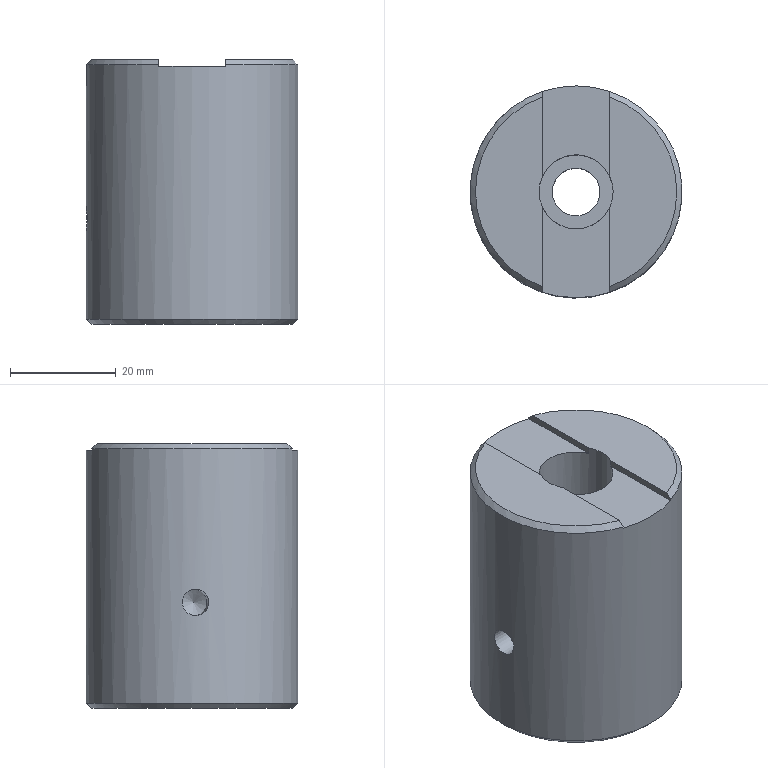Part | STEP file | gslz 2016.10.28-6_id170_x_t | 1 solid | 18 faces | box 40 x 40 x 50 mm | volume 56993 mm3 | plane 10 | cylinder 4 | cone 4 | commonest cylinder face diameters 5 x1 9 x1 14 x1 40 x1
STEP:
#1=CARTESIAN_POINT('',(-259.,150.,-0.007538));
#2=VERTEX_POINT('',#1);
#3=CARTESIAN_POINT('',(-240.,150.,-0.007538));
#4=DIRECTION('',(0.,0.,1.));
#5=DIRECTION('',(-1.,0.,0.));
#6=AXIS2_PLACEMENT_3D('',#3,#4,#5);
#7=CIRCLE('',#6,19.);
#8=EDGE_CURVE('',#2,#2,#7,.T.);
#9=ORIENTED_EDGE('',*,*,#8,.F.);
#10=EDGE_LOOP('',(#9));
#11=FACE_BOUND('',#10,.T.);
#12=CARTESIAN_POINT('',(-235.5,150.,-0.007538));
#13=VERTEX_POINT('',#12);
#14=CARTESIAN_POINT('',(-240.,150.,-0.007538));
#15=DIRECTION('',(0.,0.,1.));
#16=DIRECTION('',(1.,0.,0.));
#17=AXIS2_PLACEMENT_3D('',#14,#15,#16);
#18=CIRCLE('',#17,4.5);
#19=EDGE_CURVE('',#13,#13,#18,.T.);
#20=ORIENTED_EDGE('',*,*,#19,.T.);
#21=EDGE_LOOP('',(#20));
#22=FACE_BOUND('',#21,.T.);
#23=CARTESIAN_POINT('',(-240.,150.,-0.007538));
#24=DIRECTION('',(0.,0.,1.));
#25=DIRECTION('',(-1.,0.,0.));
#26=AXIS2_PLACEMENT_3D('',#23,#24,#25);
#27=PLANE('',#26);
#28=ADVANCED_FACE('',(#11,#22),#27,.F.);
#29=CARTESIAN_POINT('',(-233.65,147.054,49.992));
#30=VERTEX_POINT('',#29);
#31=CARTESIAN_POINT('',(-233.65,132.093,49.992));
#32=VERTEX_POINT('',#31);
#33=CARTESIAN_POINT('',(-233.65,150.,49.992));
#34=DIRECTION('',(0.,-1.,0.));
#35=VECTOR('',#34,1.);
#36=LINE('',#33,#35);
#37=EDGE_CURVE('',#30,#32,#36,.T.);
#38=ORIENTED_EDGE('',*,*,#37,.T.);
#39=CARTESIAN_POINT('',(-233.65,167.907,49.992));
#40=VERTEX_POINT('',#39);
#41=CARTESIAN_POINT('',(-240.,150.,49.992));
#42=DIRECTION('',(0.,0.,-1.));
#43=DIRECTION('',(-1.,0.,0.));
#44=AXIS2_PLACEMENT_3D('',#41,#42,#43);
#45=CIRCLE('',#44,19.);
#46=EDGE_CURVE('',#40,#32,#45,.T.);
#47=ORIENTED_EDGE('',*,*,#46,.F.);
#48=CARTESIAN_POINT('',(-233.65,152.946,49.992));
#49=VERTEX_POINT('',#48);
#50=CARTESIAN_POINT('',(-233.65,150.,49.992));
#51=DIRECTION('',(0.,-1.,0.));
#52=VECTOR('',#51,1.);
#53=LINE('',#50,#52);
#54=EDGE_CURVE('',#40,#49,#53,.T.);
#55=ORIENTED_EDGE('',*,*,#54,.T.);
#56=CARTESIAN_POINT('',(-240.,150.,49.992));
#57=DIRECTION('',(0.,0.,1.));
#58=DIRECTION('',(1.,0.,0.));
#59=AXIS2_PLACEMENT_3D('',#56,#57,#58);
#60=CIRCLE('',#59,7.);
#61=EDGE_CURVE('',#30,#49,#60,.T.);
#62=ORIENTED_EDGE('',*,*,#61,.F.);
#63=EDGE_LOOP('',(#38,#47,#55,#62));
#64=FACE_OUTER_BOUND('',#63,.T.);
#65=CARTESIAN_POINT('',(-240.,150.,49.992));
#66=DIRECTION('',(0.,0.,1.));
#67=DIRECTION('',(-1.,0.,0.));
#68=AXIS2_PLACEMENT_3D('',#65,#66,#67);
#69=PLANE('',#68);
#70=ADVANCED_FACE('',(#64),#69,.T.);
#71=CARTESIAN_POINT('',(-246.35,152.946,49.992));
#72=VERTEX_POINT('',#71);
#73=CARTESIAN_POINT('',(-246.35,167.907,49.992));
#74=VERTEX_POINT('',#73);
#75=CARTESIAN_POINT('',(-246.35,150.,49.992));
#76=DIRECTION('',(0.,1.,0.));
#77=VECTOR('',#76,1.);
#78=LINE('',#75,#77);
#79=EDGE_CURVE('',#72,#74,#78,.T.);
#80=ORIENTED_EDGE('',*,*,#79,.T.);
#81=CARTESIAN_POINT('',(-246.35,132.093,49.992));
#82=VERTEX_POINT('',#81);
#83=CARTESIAN_POINT('',(-240.,150.,49.992));
#84=DIRECTION('',(0.,0.,-1.));
#85=DIRECTION('',(-1.,0.,0.));
#86=AXIS2_PLACEMENT_3D('',#83,#84,#85);
#87=CIRCLE('',#86,19.);
#88=EDGE_CURVE('',#82,#74,#87,.T.);
#89=ORIENTED_EDGE('',*,*,#88,.F.);
#90=CARTESIAN_POINT('',(-246.35,147.054,49.992));
#91=VERTEX_POINT('',#90);
#92=CARTESIAN_POINT('',(-246.35,150.,49.992));
#93=DIRECTION('',(0.,1.,0.));
#94=VECTOR('',#93,1.);
#95=LINE('',#92,#94);
#96=EDGE_CURVE('',#82,#91,#95,.T.);
#97=ORIENTED_EDGE('',*,*,#96,.T.);
#98=CARTESIAN_POINT('',(-240.,150.,49.992));
#99=DIRECTION('',(0.,0.,1.));
#100=DIRECTION('',(1.,0.,0.));
#101=AXIS2_PLACEMENT_3D('',#98,#99,#100);
#102=CIRCLE('',#101,7.);
#103=EDGE_CURVE('',#72,#91,#102,.T.);
#104=ORIENTED_EDGE('',*,*,#103,.F.);
#105=EDGE_LOOP('',(#80,#89,#97,#104));
#106=FACE_OUTER_BOUND('',#105,.T.);
#107=CARTESIAN_POINT('',(-240.,150.,49.992));
#108=DIRECTION('',(0.,0.,1.));
#109=DIRECTION('',(-1.,0.,0.));
#110=AXIS2_PLACEMENT_3D('',#107,#108,#109);
#111=PLANE('',#110);
#112=ADVANCED_FACE('',(#106),#111,.T.);
#113=ORIENTED_EDGE('',*,*,#96,.F.);
#114=CARTESIAN_POINT('',(-246.35,131.035,48.992));
#115=VERTEX_POINT('',#114);
#116=CARTESIAN_POINT('',(-246.35,131.035,48.992));
#117=CARTESIAN_POINT('',(-246.35,131.387,49.326));
#118=CARTESIAN_POINT('',(-246.35,131.739,49.66));
#119=CARTESIAN_POINT('',(-246.35,132.093,49.992));
#120=B_SPLINE_CURVE_WITH_KNOTS('',3,(#116,#117,#118,#119),.UNSPECIFIED.,.F.,.F.,(4,4),(0.,1.),.UNSPECIFIED.);
#121=EDGE_CURVE('',#115,#82,#120,.T.);
#122=ORIENTED_EDGE('',*,*,#121,.F.);
#123=CARTESIAN_POINT('',(-246.35,131.035,48.722));
#124=VERTEX_POINT('',#123);
#125=CARTESIAN_POINT('',(-246.35,131.035,-35.008));
#126=DIRECTION('',(0.,0.,1.));
#127=VECTOR('',#126,1.);
#128=LINE('',#125,#127);
#129=EDGE_CURVE('',#124,#115,#128,.T.);
#130=ORIENTED_EDGE('',*,*,#129,.F.);
#131=CARTESIAN_POINT('',(-246.35,147.054,48.722));
#132=VERTEX_POINT('',#131);
#133=CARTESIAN_POINT('',(-246.35,1261.518,48.722));
#134=DIRECTION('',(0.,1.,0.));
#135=VECTOR('',#134,1.);
#136=LINE('',#133,#135);
#137=EDGE_CURVE('',#124,#132,#136,.T.);
#138=ORIENTED_EDGE('',*,*,#137,.T.);
#139=CARTESIAN_POINT('',(-246.35,147.054,39.992));
#140=DIRECTION('',(0.,0.,-1.));
#141=VECTOR('',#140,1.);
#142=LINE('',#139,#141);
#143=EDGE_CURVE('',#91,#132,#142,.T.);
#144=ORIENTED_EDGE('',*,*,#143,.F.);
#145=EDGE_LOOP('',(#113,#122,#130,#138,#144));
#146=FACE_OUTER_BOUND('',#145,.T.);
#147=CARTESIAN_POINT('',(-246.35,1261.518,124.992));
#148=DIRECTION('',(-1.,0.,0.));
#149=DIRECTION('',(0.,0.,-1.));
#150=AXIS2_PLACEMENT_3D('',#147,#148,#149);
#151=PLANE('',#150);
#152=ADVANCED_FACE('',(#146),#151,.F.);
#153=ORIENTED_EDGE('',*,*,#54,.F.);
#154=CARTESIAN_POINT('',(-233.65,168.965,48.992));
#155=VERTEX_POINT('',#154);
#156=CARTESIAN_POINT('',(-233.65,168.965,48.992));
#157=CARTESIAN_POINT('',(-233.65,168.613,49.326));
#158=CARTESIAN_POINT('',(-233.65,168.261,49.66));
#159=CARTESIAN_POINT('',(-233.65,167.907,49.992));
#160=B_SPLINE_CURVE_WITH_KNOTS('',3,(#156,#157,#158,#159),.UNSPECIFIED.,.F.,.F.,(4,4),(0.,1.),.UNSPECIFIED.);
#161=EDGE_CURVE('',#155,#40,#160,.T.);
#162=ORIENTED_EDGE('',*,*,#161,.F.);
#163=CARTESIAN_POINT('',(-233.65,168.965,48.722));
#164=VERTEX_POINT('',#163);
#165=CARTESIAN_POINT('',(-233.65,168.965,-35.008));
#166=DIRECTION('',(0.,0.,1.));
#167=VECTOR('',#166,1.);
#168=LINE('',#165,#167);
#169=EDGE_CURVE('',#164,#155,#168,.T.);
#170=ORIENTED_EDGE('',*,*,#169,.F.);
#171=CARTESIAN_POINT('',(-233.65,152.946,48.722));
#172=VERTEX_POINT('',#171);
#173=CARTESIAN_POINT('',(-233.65,-113.507,48.722));
#174=DIRECTION('',(0.,-1.,0.));
#175=VECTOR('',#174,1.);
#176=LINE('',#173,#175);
#177=EDGE_CURVE('',#164,#172,#176,.T.);
#178=ORIENTED_EDGE('',*,*,#177,.T.);
#179=CARTESIAN_POINT('',(-233.65,152.946,39.992));
#180=DIRECTION('',(0.,0.,-1.));
#181=VECTOR('',#180,1.);
#182=LINE('',#179,#181);
#183=EDGE_CURVE('',#49,#172,#182,.T.);
#184=ORIENTED_EDGE('',*,*,#183,.F.);
#185=EDGE_LOOP('',(#153,#162,#170,#178,#184));
#186=FACE_OUTER_BOUND('',#185,.T.);
#187=CARTESIAN_POINT('',(-233.65,-113.507,124.992));
#188=DIRECTION('',(1.,0.,0.));
#189=DIRECTION('',(0.,0.,1.));
#190=AXIS2_PLACEMENT_3D('',#187,#188,#189);
#191=PLANE('',#190);
#192=ADVANCED_FACE('',(#186),#191,.F.);
#193=CARTESIAN_POINT('',(-246.35,152.946,48.722));
#194=VERTEX_POINT('',#193);
#195=CARTESIAN_POINT('',(-240.,150.,48.722));
#196=DIRECTION('',(0.,0.,-1.));
#197=DIRECTION('',(-1.,0.,0.));
#198=AXIS2_PLACEMENT_3D('',#195,#196,#197);
#199=CIRCLE('',#198,7.);
#200=EDGE_CURVE('',#194,#172,#199,.T.);
#201=ORIENTED_EDGE('',*,*,#200,.T.);
#202=ORIENTED_EDGE('',*,*,#177,.F.);
#203=CARTESIAN_POINT('',(-246.35,168.965,48.722));
#204=VERTEX_POINT('',#203);
#205=CARTESIAN_POINT('',(-240.,150.,48.722));
#206=DIRECTION('',(0.,0.,1.));
#207=DIRECTION('',(-1.,0.,0.));
#208=AXIS2_PLACEMENT_3D('',#205,#206,#207);
#209=CIRCLE('',#208,20.);
#210=EDGE_CURVE('',#164,#204,#209,.T.);
#211=ORIENTED_EDGE('',*,*,#210,.T.);
#212=CARTESIAN_POINT('',(-246.35,1261.518,48.722));
#213=DIRECTION('',(0.,1.,0.));
#214=VECTOR('',#213,1.);
#215=LINE('',#212,#214);
#216=EDGE_CURVE('',#194,#204,#215,.T.);
#217=ORIENTED_EDGE('',*,*,#216,.F.);
#218=EDGE_LOOP('',(#201,#202,#211,#217));
#219=FACE_OUTER_BOUND('',#218,.T.);
#220=CARTESIAN_POINT('',(-233.65,574.005,48.722));
#221=DIRECTION('',(0.,0.,1.));
#222=DIRECTION('',(-1.,0.,0.));
#223=AXIS2_PLACEMENT_3D('',#220,#221,#222);
#224=PLANE('',#223);
#225=ADVANCED_FACE('',(#219),#224,.T.);
#226=CARTESIAN_POINT('',(-260.,150.,0.9925));
#227=VERTEX_POINT('',#226);
#228=CARTESIAN_POINT('',(-240.,150.,0.9925));
#229=DIRECTION('',(0.,0.,-1.));
#230=DIRECTION('',(-1.,0.,0.));
#231=AXIS2_PLACEMENT_3D('',#228,#229,#230);
#232=CIRCLE('',#231,20.);
#233=EDGE_CURVE('',#227,#227,#232,.T.);
#234=ORIENTED_EDGE('',*,*,#233,.F.);
#235=EDGE_LOOP('',(#234));
#236=FACE_BOUND('',#235,.T.);
#237=CARTESIAN_POINT('',(-233.65,131.035,48.992));
#238=VERTEX_POINT('',#237);
#239=CARTESIAN_POINT('',(-233.65,131.035,48.722));
#240=VERTEX_POINT('',#239);
#241=CARTESIAN_POINT('',(-233.65,131.035,-35.008));
#242=DIRECTION('',(0.,0.,-1.));
#243=VECTOR('',#242,1.);
#244=LINE('',#241,#243);
#245=EDGE_CURVE('',#238,#240,#244,.T.);
#246=ORIENTED_EDGE('',*,*,#245,.T.);
#247=CARTESIAN_POINT('',(-240.,150.,48.722));
#248=DIRECTION('',(0.,0.,1.));
#249=DIRECTION('',(-1.,0.,0.));
#250=AXIS2_PLACEMENT_3D('',#247,#248,#249);
#251=CIRCLE('',#250,20.);
#252=EDGE_CURVE('',#124,#240,#251,.T.);
#253=ORIENTED_EDGE('',*,*,#252,.F.);
#254=ORIENTED_EDGE('',*,*,#129,.T.);
#255=CARTESIAN_POINT('',(-246.35,168.965,48.992));
#256=VERTEX_POINT('',#255);
#257=CARTESIAN_POINT('',(-240.,150.,48.992));
#258=DIRECTION('',(0.,0.,1.));
#259=DIRECTION('',(-1.,0.,0.));
#260=AXIS2_PLACEMENT_3D('',#257,#258,#259);
#261=CIRCLE('',#260,20.);
#262=EDGE_CURVE('',#256,#115,#261,.T.);
#263=ORIENTED_EDGE('',*,*,#262,.F.);
#264=CARTESIAN_POINT('',(-246.35,168.965,48.857));
#265=DIRECTION('',(0.,0.,-1.));
#266=VECTOR('',#265,1.);
#267=LINE('',#264,#266);
#268=EDGE_CURVE('',#256,#204,#267,.T.);
#269=ORIENTED_EDGE('',*,*,#268,.T.);
#270=ORIENTED_EDGE('',*,*,#210,.F.);
#271=ORIENTED_EDGE('',*,*,#169,.T.);
#272=CARTESIAN_POINT('',(-240.,150.,48.992));
#273=DIRECTION('',(0.,0.,1.));
#274=DIRECTION('',(-1.,0.,0.));
#275=AXIS2_PLACEMENT_3D('',#272,#273,#274);
#276=CIRCLE('',#275,20.);
#277=EDGE_CURVE('',#238,#155,#276,.T.);
#278=ORIENTED_EDGE('',*,*,#277,.F.);
#279=EDGE_LOOP('',(#246,#253,#254,#263,#269,#270,#271,#278));
#280=FACE_BOUND('',#279,.T.);
#281=CARTESIAN_POINT('',(-259.98,149.117,17.502));
#282=VERTEX_POINT('',#281);
#283=CARTESIAN_POINT('',(-259.98,149.117,17.502));
#284=CARTESIAN_POINT('',(-259.993,149.394,17.478));
#285=CARTESIAN_POINT('',(-259.999,149.679,17.5));
#286=CARTESIAN_POINT('',(-260.,149.949,17.568));
#287=CARTESIAN_POINT('',(-260.001,150.218,17.637));
#288=CARTESIAN_POINT('',(-259.996,150.48,17.752));
#289=CARTESIAN_POINT('',(-259.987,150.713,17.904));
#290=CARTESIAN_POINT('',(-259.979,150.946,18.058));
#291=CARTESIAN_POINT('',(-259.967,151.156,18.253));
#292=CARTESIAN_POINT('',(-259.956,151.326,18.475));
#293=CARTESIAN_POINT('',(-259.945,151.496,18.698));
#294=CARTESIAN_POINT('',(-259.934,151.631,18.953));
#295=CARTESIAN_POINT('',(-259.926,151.718,19.22));
#296=CARTESIAN_POINT('',(-259.919,151.805,19.486));
#297=CARTESIAN_POINT('',(-259.915,151.847,19.771));
#298=CARTESIAN_POINT('',(-259.915,151.84,20.051));
#299=CARTESIAN_POINT('',(-259.916,151.834,20.328));
#300=CARTESIAN_POINT('',(-259.921,151.779,20.609));
#301=CARTESIAN_POINT('',(-259.929,151.681,20.869));
#302=CARTESIAN_POINT('',(-259.937,151.584,21.129));
#303=CARTESIAN_POINT('',(-259.949,151.44,21.376));
#304=CARTESIAN_POINT('',(-259.96,151.262,21.59));
#305=CARTESIAN_POINT('',(-259.971,151.083,21.805));
#306=CARTESIAN_POINT('',(-259.983,150.864,21.992));
#307=CARTESIAN_POINT('',(-259.99,150.624,22.136));
#308=CARTESIAN_POINT('',(-259.998,150.384,22.28));
#309=CARTESIAN_POINT('',(-260.002,150.114,22.385));
#310=CARTESIAN_POINT('',(-259.999,149.839,22.441));
#311=CARTESIAN_POINT('',(-259.997,149.566,22.498));
#312=CARTESIAN_POINT('',(-259.989,149.279,22.507));
#313=CARTESIAN_POINT('',(-259.975,149.003,22.47));
#314=CARTESIAN_POINT('',(-259.961,148.728,22.433));
#315=CARTESIAN_POINT('',(-259.942,148.456,22.348));
#316=CARTESIAN_POINT('',(-259.92,148.209,22.223));
#317=CARTESIAN_POINT('',(-259.897,147.961,22.097));
#318=CARTESIAN_POINT('',(-259.872,147.732,21.927));
#319=CARTESIAN_POINT('',(-259.848,147.54,21.727));
#320=CARTESIAN_POINT('',(-259.824,147.346,21.525));
#321=CARTESIAN_POINT('',(-259.801,147.185,21.287));
#322=CARTESIAN_POINT('',(-259.784,147.069,21.032));
#323=CARTESIAN_POINT('',(-259.767,146.953,20.777));
#324=CARTESIAN_POINT('',(-259.755,146.879,20.498));
#325=CARTESIAN_POINT('',(-259.751,146.854,20.219));
#326=CARTESIAN_POINT('',(-259.747,146.829,19.942));
#327=CARTESIAN_POINT('',(-259.751,146.851,19.656));
#328=CARTESIAN_POINT('',(-259.761,146.918,19.386));
#329=CARTESIAN_POINT('',(-259.771,146.985,19.117));
#330=CARTESIAN_POINT('',(-259.789,147.099,18.855));
#331=CARTESIAN_POINT('',(-259.81,147.25,18.623));
#332=CARTESIAN_POINT('',(-259.831,147.402,18.39));
#333=CARTESIAN_POINT('',(-259.856,147.596,18.18));
#334=CARTESIAN_POINT('',(-259.88,147.817,18.01));
#335=CARTESIAN_POINT('',(-259.905,148.038,17.839));
#336=CARTESIAN_POINT('',(-259.929,148.293,17.704));
#337=CARTESIAN_POINT('',(-259.948,148.559,17.617));
#338=CARTESIAN_POINT('',(-259.961,148.739,17.558));
#339=CARTESIAN_POINT('',(-259.972,148.927,17.519));
#340=CARTESIAN_POINT('',(-259.98,149.117,17.502));
#341=B_SPLINE_CURVE_WITH_KNOTS('',3,(#283,#284,#285,#286,#287,#288,#289,#290,#291,#292,#293,#294,#295,#296,#297,#298,#299,#300,#301,#302,#303,#304,#305,#306,#307,#308,#309,#310,#311,#312,#313,#314,#315,#316,#317,#318,#319,#320,#321,#322,#323,#324,#325,#326,#327,#328,#329,#330,#331,#332,#333,#334,#335,#336,#337,#338,#339,#340),.UNSPECIFIED.,.T.,.F.,(1,3,3,3,3,3,3,3,3,3,3,3,3,3,3,3,3,3,3,3,3,1),(-0.0362,0.,0.05335,0.1067,0.1602,0.2141,0.2678,0.3211,0.3744,0.4281,0.4819,0.5355,0.5887,0.6421,0.6959,0.7497,0.8031,0.8564,0.9099,0.9638,1.,1.053),.UNSPECIFIED.);
#342=EDGE_CURVE('',#282,#282,#341,.T.);
#343=ORIENTED_EDGE('',*,*,#342,.T.);
#344=EDGE_LOOP('',(#343));
#345=FACE_BOUND('',#344,.T.);
#346=CARTESIAN_POINT('',(-240.,150.,-35.008));
#347=DIRECTION('',(0.,0.,1.));
#348=DIRECTION('',(1.,0.,0.));
#349=AXIS2_PLACEMENT_3D('',#346,#347,#348);
#350=CYLINDRICAL_SURFACE('',#349,20.);
#351=ADVANCED_FACE('',(#236,#280,#345),#350,.T.);
#352=ORIENTED_EDGE('',*,*,#216,.T.);
#353=ORIENTED_EDGE('',*,*,#268,.F.);
#354=CARTESIAN_POINT('',(-246.35,167.907,49.992));
#355=CARTESIAN_POINT('',(-246.35,168.261,49.66));
#356=CARTESIAN_POINT('',(-246.35,168.613,49.326));
#357=CARTESIAN_POINT('',(-246.35,168.965,48.992));
#358=B_SPLINE_CURVE_WITH_KNOTS('',3,(#354,#355,#356,#357),.UNSPECIFIED.,.F.,.F.,(4,4),(0.,1.),.UNSPECIFIED.);
#359=EDGE_CURVE('',#74,#256,#358,.T.);
#360=ORIENTED_EDGE('',*,*,#359,.F.);
#361=ORIENTED_EDGE('',*,*,#79,.F.);
#362=CARTESIAN_POINT('',(-246.35,152.946,39.992));
#363=DIRECTION('',(0.,0.,1.));
#364=VECTOR('',#363,1.);
#365=LINE('',#362,#364);
#366=EDGE_CURVE('',#194,#72,#365,.T.);
#367=ORIENTED_EDGE('',*,*,#366,.F.);
#368=EDGE_LOOP('',(#352,#353,#360,#361,#367));
#369=FACE_OUTER_BOUND('',#368,.T.);
#370=CARTESIAN_POINT('',(-246.35,1261.518,124.992));
#371=DIRECTION('',(-1.,0.,0.));
#372=DIRECTION('',(0.,0.,-1.));
#373=AXIS2_PLACEMENT_3D('',#370,#371,#372);
#374=PLANE('',#373);
#375=ADVANCED_FACE('',(#369),#374,.F.);
#376=CARTESIAN_POINT('',(-233.65,147.054,48.722));
#377=VERTEX_POINT('',#376);
#378=CARTESIAN_POINT('',(-233.65,-113.507,48.722));
#379=DIRECTION('',(0.,-1.,0.));
#380=VECTOR('',#379,1.);
#381=LINE('',#378,#380);
#382=EDGE_CURVE('',#377,#240,#381,.T.);
#383=ORIENTED_EDGE('',*,*,#382,.T.);
#384=ORIENTED_EDGE('',*,*,#245,.F.);
#385=CARTESIAN_POINT('',(-233.65,132.093,49.992));
#386=CARTESIAN_POINT('',(-233.65,131.739,49.66));
#387=CARTESIAN_POINT('',(-233.65,131.387,49.326));
#388=CARTESIAN_POINT('',(-233.65,131.035,48.992));
#389=B_SPLINE_CURVE_WITH_KNOTS('',3,(#385,#386,#387,#388),.UNSPECIFIED.,.F.,.F.,(4,4),(0.,1.),.UNSPECIFIED.);
#390=EDGE_CURVE('',#32,#238,#389,.T.);
#391=ORIENTED_EDGE('',*,*,#390,.F.);
#392=ORIENTED_EDGE('',*,*,#37,.F.);
#393=CARTESIAN_POINT('',(-233.65,147.054,39.992));
#394=DIRECTION('',(0.,0.,1.));
#395=VECTOR('',#394,1.);
#396=LINE('',#393,#395);
#397=EDGE_CURVE('',#377,#30,#396,.T.);
#398=ORIENTED_EDGE('',*,*,#397,.F.);
#399=EDGE_LOOP('',(#383,#384,#391,#392,#398));
#400=FACE_OUTER_BOUND('',#399,.T.);
#401=CARTESIAN_POINT('',(-233.65,-113.507,124.992));
#402=DIRECTION('',(1.,0.,0.));
#403=DIRECTION('',(0.,0.,1.));
#404=AXIS2_PLACEMENT_3D('',#401,#402,#403);
#405=PLANE('',#404);
#406=ADVANCED_FACE('',(#400),#405,.F.);
#407=CARTESIAN_POINT('',(-240.,150.,48.722));
#408=DIRECTION('',(0.,0.,-1.));
#409=DIRECTION('',(-1.,0.,0.));
#410=AXIS2_PLACEMENT_3D('',#407,#408,#409);
#411=CIRCLE('',#410,7.);
#412=EDGE_CURVE('',#377,#132,#411,.T.);
#413=ORIENTED_EDGE('',*,*,#412,.T.);
#414=ORIENTED_EDGE('',*,*,#137,.F.);
#415=ORIENTED_EDGE('',*,*,#252,.T.);
#416=ORIENTED_EDGE('',*,*,#382,.F.);
#417=EDGE_LOOP('',(#413,#414,#415,#416));
#418=FACE_OUTER_BOUND('',#417,.T.);
#419=CARTESIAN_POINT('',(-233.65,574.005,48.722));
#420=DIRECTION('',(0.,0.,1.));
#421=DIRECTION('',(-1.,0.,0.));
#422=AXIS2_PLACEMENT_3D('',#419,#420,#421);
#423=PLANE('',#422);
#424=ADVANCED_FACE('',(#418),#423,.T.);
#425=CARTESIAN_POINT('',(-249.912,147.17,19.992));
#426=VERTEX_POINT('',#425);
#427=CARTESIAN_POINT('',(-249.994,149.668,19.992));
#428=DIRECTION('',(0.9995,0.03316,0.));
#429=DIRECTION('',(0.03316,-0.9995,0.));
#430=AXIS2_PLACEMENT_3D('',#427,#428,#429);
#431=CIRCLE('',#430,2.5);
#432=EDGE_CURVE('',#426,#426,#431,.T.);
#433=ORIENTED_EDGE('',*,*,#432,.F.);
#434=EDGE_LOOP('',(#433));
#435=FACE_BOUND('',#434,.T.);
#436=CARTESIAN_POINT('',(-248.493,149.718,19.992));
#437=VERTEX_POINT('',#436);
#438=VERTEX_LOOP('',#437);
#439=FACE_BOUND('',#438,.T.);
#440=CARTESIAN_POINT('',(-249.994,149.668,19.992));
#441=DIRECTION('',(-0.9995,-0.03316,0.));
#442=DIRECTION('',(-0.03316,0.9995,0.));
#443=AXIS2_PLACEMENT_3D('',#440,#441,#442);
#444=CONICAL_SURFACE('',#443,2.5,59.);
#445=ADVANCED_FACE('',(#435,#439),#444,.F.);
#446=ORIENTED_EDGE('',*,*,#342,.F.);
#447=EDGE_LOOP('',(#446));
#448=FACE_BOUND('',#447,.T.);
#449=ORIENTED_EDGE('',*,*,#432,.T.);
#450=EDGE_LOOP('',(#449));
#451=FACE_BOUND('',#450,.T.);
#452=CARTESIAN_POINT('',(-264.986,149.171,19.992));
#453=DIRECTION('',(0.9995,0.03316,0.));
#454=DIRECTION('',(-0.03316,0.9995,0.));
#455=AXIS2_PLACEMENT_3D('',#452,#453,#454);
#456=CYLINDRICAL_SURFACE('',#455,2.5);
#457=ADVANCED_FACE('',(#448,#451),#456,.F.);
#458=ORIENTED_EDGE('',*,*,#8,.T.);
#459=EDGE_LOOP('',(#458));
#460=FACE_BOUND('',#459,.T.);
#461=ORIENTED_EDGE('',*,*,#233,.T.);
#462=EDGE_LOOP('',(#461));
#463=FACE_BOUND('',#462,.T.);
#464=CARTESIAN_POINT('',(-240.,150.,0.9925));
#465=DIRECTION('',(0.,0.,1.));
#466=DIRECTION('',(1.,0.,0.));
#467=AXIS2_PLACEMENT_3D('',#464,#465,#466);
#468=CONICAL_SURFACE('',#467,20.,45.);
#469=ADVANCED_FACE('',(#460,#463),#468,.T.);
#470=ORIENTED_EDGE('',*,*,#390,.T.);
#471=ORIENTED_EDGE('',*,*,#277,.T.);
#472=ORIENTED_EDGE('',*,*,#161,.T.);
#473=ORIENTED_EDGE('',*,*,#46,.T.);
#474=EDGE_LOOP('',(#470,#471,#472,#473));
#475=FACE_OUTER_BOUND('',#474,.T.);
#476=CARTESIAN_POINT('',(-240.,150.,48.992));
#477=DIRECTION('',(0.,0.,-1.));
#478=DIRECTION('',(-1.,0.,0.));
#479=AXIS2_PLACEMENT_3D('',#476,#477,#478);
#480=CONICAL_SURFACE('',#479,20.,45.);
#481=ADVANCED_FACE('',(#475),#480,.T.);
#482=ORIENTED_EDGE('',*,*,#359,.T.);
#483=ORIENTED_EDGE('',*,*,#262,.T.);
#484=ORIENTED_EDGE('',*,*,#121,.T.);
#485=ORIENTED_EDGE('',*,*,#88,.T.);
#486=EDGE_LOOP('',(#482,#483,#484,#485));
#487=FACE_OUTER_BOUND('',#486,.T.);
#488=CARTESIAN_POINT('',(-240.,150.,48.992));
#489=DIRECTION('',(0.,0.,-1.));
#490=DIRECTION('',(-1.,0.,0.));
#491=AXIS2_PLACEMENT_3D('',#488,#489,#490);
#492=CONICAL_SURFACE('',#491,20.,45.);
#493=ADVANCED_FACE('',(#487),#492,.T.);
#494=CARTESIAN_POINT('',(-233.,150.,28.992));
#495=VERTEX_POINT('',#494);
#496=CARTESIAN_POINT('',(-240.,150.,28.992));
#497=DIRECTION('',(0.,0.,-1.));
#498=DIRECTION('',(1.,0.,0.));
#499=AXIS2_PLACEMENT_3D('',#496,#497,#498);
#500=CIRCLE('',#499,7.);
#501=EDGE_CURVE('',#495,#495,#500,.T.);
#502=ORIENTED_EDGE('',*,*,#501,.T.);
#503=EDGE_LOOP('',(#502));
#504=FACE_BOUND('',#503,.T.);
#505=ORIENTED_EDGE('',*,*,#200,.F.);
#506=ORIENTED_EDGE('',*,*,#366,.T.);
#507=ORIENTED_EDGE('',*,*,#103,.T.);
#508=ORIENTED_EDGE('',*,*,#143,.T.);
#509=ORIENTED_EDGE('',*,*,#412,.F.);
#510=ORIENTED_EDGE('',*,*,#397,.T.);
#511=ORIENTED_EDGE('',*,*,#61,.T.);
#512=ORIENTED_EDGE('',*,*,#183,.T.);
#513=EDGE_LOOP('',(#505,#506,#507,#508,#509,#510,#511,#512));
#514=FACE_BOUND('',#513,.T.);
#515=CARTESIAN_POINT('',(-240.,150.,39.992));
#516=DIRECTION('',(0.,0.,-1.));
#517=DIRECTION('',(-1.,0.,0.));
#518=AXIS2_PLACEMENT_3D('',#515,#516,#517);
#519=CYLINDRICAL_SURFACE('',#518,7.);
#520=ADVANCED_FACE('',(#504,#514),#519,.F.);
#521=ORIENTED_EDGE('',*,*,#19,.F.);
#522=EDGE_LOOP('',(#521));
#523=FACE_BOUND('',#522,.T.);
#524=CARTESIAN_POINT('',(-235.5,150.,28.992));
#525=VERTEX_POINT('',#524);
#526=CARTESIAN_POINT('',(-240.,150.,28.992));
#527=DIRECTION('',(0.,0.,-1.));
#528=DIRECTION('',(1.,0.,0.));
#529=AXIS2_PLACEMENT_3D('',#526,#527,#528);
#530=CIRCLE('',#529,4.5);
#531=EDGE_CURVE('',#525,#525,#530,.T.);
#532=ORIENTED_EDGE('',*,*,#531,.F.);
#533=EDGE_LOOP('',(#532));
#534=FACE_BOUND('',#533,.T.);
#535=CARTESIAN_POINT('',(-240.,150.,-0.007538));
#536=DIRECTION('',(0.,0.,-1.));
#537=DIRECTION('',(-1.,0.,0.));
#538=AXIS2_PLACEMENT_3D('',#535,#536,#537);
#539=CYLINDRICAL_SURFACE('',#538,4.5);
#540=ADVANCED_FACE('',(#523,#534),#539,.F.);
#541=ORIENTED_EDGE('',*,*,#531,.T.);
#542=EDGE_LOOP('',(#541));
#543=FACE_BOUND('',#542,.T.);
#544=ORIENTED_EDGE('',*,*,#501,.F.);
#545=EDGE_LOOP('',(#544));
#546=FACE_BOUND('',#545,.T.);
#547=CARTESIAN_POINT('',(-240.,150.,28.992));
#548=DIRECTION('',(0.,0.,-1.));
#549=DIRECTION('',(-1.,0.,0.));
#550=AXIS2_PLACEMENT_3D('',#547,#548,#549);
#551=PLANE('',#550);
#552=ADVANCED_FACE('',(#543,#546),#551,.F.);
#553=CLOSED_SHELL('',(#28,#70,#112,#152,#192,#225,#351,#375,#406,#424,#445,#457,#469,#481,#493,#520,#540,#552));
#554=MANIFOLD_SOLID_BREP('',#553);
#555=(LENGTH_UNIT()NAMED_UNIT(*)SI_UNIT(.MILLI.,.METRE.));
#556=UNCERTAINTY_MEASURE_WITH_UNIT(LENGTH_MEASURE(0.0508),#555,'','');
#557=(NAMED_UNIT(*)PLANE_ANGLE_UNIT()SI_UNIT($,.RADIAN.));
#558=PLANE_ANGLE_MEASURE_WITH_UNIT(PLANE_ANGLE_MEASURE(0.01745),#557);
#559=DIMENSIONAL_EXPONENTS(0.,0.,0.,0.,0.,0.,0.);
#560=(CONVERSION_BASED_UNIT('DEGREE',#558)NAMED_UNIT(#559)PLANE_ANGLE_UNIT());
#561=(NAMED_UNIT(*)SI_UNIT($,.STERADIAN.)SOLID_ANGLE_UNIT());
#562=(GEOMETRIC_REPRESENTATION_CONTEXT(3)GLOBAL_UNCERTAINTY_ASSIGNED_CONTEXT((#556))GLOBAL_UNIT_ASSIGNED_CONTEXT((#555,#560,#561))REPRESENTATION_CONTEXT('',''));
#563=ADVANCED_BREP_SHAPE_REPRESENTATION('',(#554),#562);